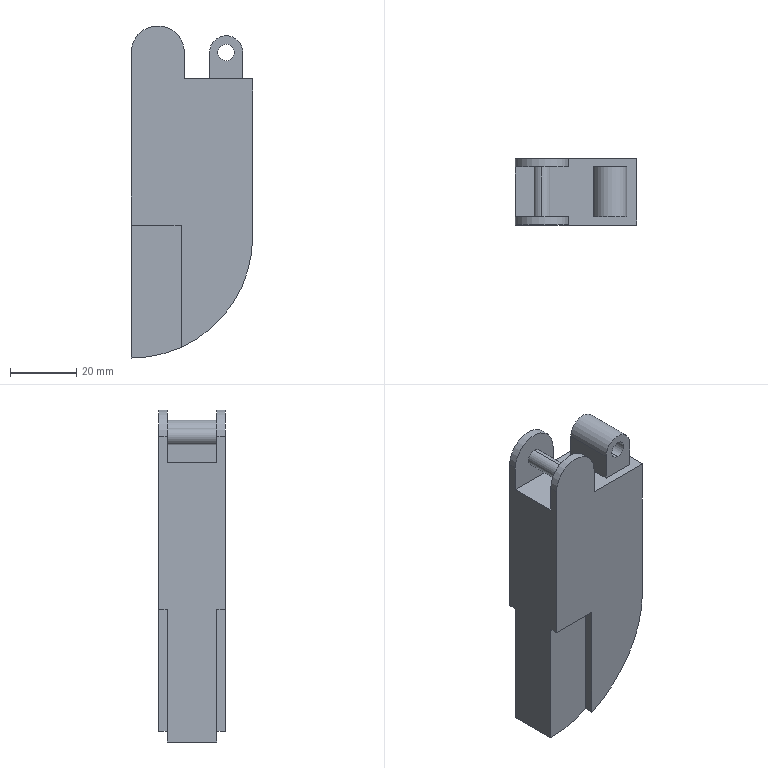Part | SolidWorks | 2 solids | 28 faces | box 36.56 x 20 x 100 mm | volume 55695 mm3 | plane 20 | cylinder 8 | commonest cylinder face diameters 5 x4 16 x2 10 x1 73.12 x1
STEP:
#1=CARTESIAN_POINT('',(8.,-7.5,-5.5));
#2=VERTEX_POINT('',#1);
#3=CARTESIAN_POINT('',(8.,-7.5,-10.5));
#4=VERTEX_POINT('',#3);
#5=CARTESIAN_POINT('',(8.,-7.5,-8.));
#6=DIRECTION('',(0.,1.,0.));
#7=DIRECTION('',(0.,0.,1.));
#8=AXIS2_PLACEMENT_3D('',#5,#6,#7);
#9=CIRCLE('',#8,2.5);
#10=EDGE_CURVE('',#2,#4,#9,.T.);
#11=ORIENTED_EDGE('',*,*,#10,.T.);
#12=CARTESIAN_POINT('',(8.,7.5,-10.5));
#13=VERTEX_POINT('',#12);
#14=CARTESIAN_POINT('',(8.,-17.071,-10.5));
#15=DIRECTION('',(0.,1.,0.));
#16=VECTOR('',#15,1000.);
#17=LINE('',#14,#16);
#18=EDGE_CURVE('',#4,#13,#17,.T.);
#19=ORIENTED_EDGE('',*,*,#18,.T.);
#20=CARTESIAN_POINT('',(8.,7.5,-5.5));
#21=VERTEX_POINT('',#20);
#22=CARTESIAN_POINT('',(8.,7.5,-8.));
#23=DIRECTION('',(0.,1.,0.));
#24=DIRECTION('',(0.,0.,1.));
#25=AXIS2_PLACEMENT_3D('',#22,#23,#24);
#26=CIRCLE('',#25,2.5);
#27=EDGE_CURVE('',#21,#13,#26,.T.);
#28=ORIENTED_EDGE('',*,*,#27,.F.);
#29=CARTESIAN_POINT('',(8.,-17.071,-5.5));
#30=DIRECTION('',(0.,1.,0.));
#31=VECTOR('',#30,1000.);
#32=LINE('',#29,#31);
#33=EDGE_CURVE('',#2,#21,#32,.T.);
#34=ORIENTED_EDGE('',*,*,#33,.F.);
#35=EDGE_LOOP('',(#11,#19,#28,#34));
#36=FACE_OUTER_BOUND('',#35,.T.);
#37=CARTESIAN_POINT('',(8.,-17.071,-8.));
#38=DIRECTION('',(0.,1.,0.));
#39=DIRECTION('',(0.,0.,1.));
#40=AXIS2_PLACEMENT_3D('',#37,#38,#39);
#41=CYLINDRICAL_SURFACE('',#40,2.5);
#42=ADVANCED_FACE('',(#36),#41,.T.);
#43=CARTESIAN_POINT('',(0.,10.,-8.));
#44=VERTEX_POINT('',#43);
#45=CARTESIAN_POINT('',(16.,10.,-8.));
#46=VERTEX_POINT('',#45);
#47=CARTESIAN_POINT('',(8.,10.,-8.));
#48=DIRECTION('',(0.,1.,0.));
#49=DIRECTION('',(0.,0.,1.));
#50=AXIS2_PLACEMENT_3D('',#47,#48,#49);
#51=CIRCLE('',#50,8.);
#52=EDGE_CURVE('',#44,#46,#51,.T.);
#53=ORIENTED_EDGE('',*,*,#52,.T.);
#54=CARTESIAN_POINT('',(16.,10.,-16.));
#55=VERTEX_POINT('',#54);
#56=CARTESIAN_POINT('',(16.,10.,-63.44));
#57=DIRECTION('',(0.,0.,1.));
#58=VECTOR('',#57,1000.);
#59=LINE('',#56,#58);
#60=EDGE_CURVE('',#55,#46,#59,.T.);
#61=ORIENTED_EDGE('',*,*,#60,.F.);
#62=CARTESIAN_POINT('',(36.56,10.,-16.));
#63=VERTEX_POINT('',#62);
#64=CARTESIAN_POINT('',(0.,10.,-16.));
#65=DIRECTION('',(-1.,0.,0.));
#66=VECTOR('',#65,1000.);
#67=LINE('',#64,#66);
#68=EDGE_CURVE('',#63,#55,#67,.T.);
#69=ORIENTED_EDGE('',*,*,#68,.F.);
#70=CARTESIAN_POINT('',(36.56,10.,-63.44));
#71=VERTEX_POINT('',#70);
#72=CARTESIAN_POINT('',(36.56,10.,0.));
#73=DIRECTION('',(0.,0.,-1.));
#74=VECTOR('',#73,1000.);
#75=LINE('',#72,#74);
#76=EDGE_CURVE('',#63,#71,#75,.T.);
#77=ORIENTED_EDGE('',*,*,#76,.T.);
#78=CARTESIAN_POINT('',(15.,10.,-96.781));
#79=VERTEX_POINT('',#78);
#80=CARTESIAN_POINT('',(0.,10.,-63.44));
#81=DIRECTION('',(0.,1.,0.));
#82=DIRECTION('',(0.,0.,1.));
#83=AXIS2_PLACEMENT_3D('',#80,#81,#82);
#84=CIRCLE('',#83,36.56);
#85=EDGE_CURVE('',#71,#79,#84,.T.);
#86=ORIENTED_EDGE('',*,*,#85,.T.);
#87=CARTESIAN_POINT('',(15.,10.,-60.));
#88=VERTEX_POINT('',#87);
#89=CARTESIAN_POINT('',(15.,10.,-100.));
#90=DIRECTION('',(0.,0.,-1.));
#91=VECTOR('',#90,1000.);
#92=LINE('',#89,#91);
#93=EDGE_CURVE('',#88,#79,#92,.T.);
#94=ORIENTED_EDGE('',*,*,#93,.F.);
#95=CARTESIAN_POINT('',(0.,10.,-60.));
#96=VERTEX_POINT('',#95);
#97=CARTESIAN_POINT('',(15.,10.,-60.));
#98=DIRECTION('',(-1.,0.,0.));
#99=VECTOR('',#98,1000.);
#100=LINE('',#97,#99);
#101=EDGE_CURVE('',#88,#96,#100,.T.);
#102=ORIENTED_EDGE('',*,*,#101,.T.);
#103=CARTESIAN_POINT('',(0.,10.,0.));
#104=DIRECTION('',(0.,0.,1.));
#105=VECTOR('',#104,1000.);
#106=LINE('',#103,#105);
#107=EDGE_CURVE('',#96,#44,#106,.T.);
#108=ORIENTED_EDGE('',*,*,#107,.T.);
#109=EDGE_LOOP('',(#53,#61,#69,#77,#86,#94,#102,#108));
#110=FACE_OUTER_BOUND('',#109,.T.);
#111=CARTESIAN_POINT('',(0.,10.,-63.44));
#112=DIRECTION('',(0.,1.,0.));
#113=DIRECTION('',(0.,0.,1.));
#114=AXIS2_PLACEMENT_3D('',#111,#112,#113);
#115=PLANE('',#114);
#116=ADVANCED_FACE('',(#110),#115,.T.);
#117=CARTESIAN_POINT('',(16.,-10.,-16.));
#118=VERTEX_POINT('',#117);
#119=CARTESIAN_POINT('',(16.,-10.,-8.));
#120=VERTEX_POINT('',#119);
#121=CARTESIAN_POINT('',(16.,-10.,-63.44));
#122=DIRECTION('',(0.,0.,1.));
#123=VECTOR('',#122,1000.);
#124=LINE('',#121,#123);
#125=EDGE_CURVE('',#118,#120,#124,.T.);
#126=ORIENTED_EDGE('',*,*,#125,.T.);
#127=CARTESIAN_POINT('',(0.,-10.,-8.));
#128=VERTEX_POINT('',#127);
#129=CARTESIAN_POINT('',(8.,-10.,-8.));
#130=DIRECTION('',(0.,-1.,0.));
#131=DIRECTION('',(0.,0.,1.));
#132=AXIS2_PLACEMENT_3D('',#129,#130,#131);
#133=CIRCLE('',#132,8.);
#134=EDGE_CURVE('',#120,#128,#133,.T.);
#135=ORIENTED_EDGE('',*,*,#134,.T.);
#136=CARTESIAN_POINT('',(0.,-10.,-60.));
#137=VERTEX_POINT('',#136);
#138=CARTESIAN_POINT('',(0.,-10.,0.));
#139=DIRECTION('',(0.,0.,1.));
#140=VECTOR('',#139,1000.);
#141=LINE('',#138,#140);
#142=EDGE_CURVE('',#137,#128,#141,.T.);
#143=ORIENTED_EDGE('',*,*,#142,.F.);
#144=CARTESIAN_POINT('',(15.,-10.,-60.));
#145=VERTEX_POINT('',#144);
#146=CARTESIAN_POINT('',(15.,-10.,-60.));
#147=DIRECTION('',(-1.,0.,0.));
#148=VECTOR('',#147,1000.);
#149=LINE('',#146,#148);
#150=EDGE_CURVE('',#145,#137,#149,.T.);
#151=ORIENTED_EDGE('',*,*,#150,.F.);
#152=CARTESIAN_POINT('',(15.,-10.,-96.781));
#153=VERTEX_POINT('',#152);
#154=CARTESIAN_POINT('',(15.,-10.,-63.44));
#155=DIRECTION('',(0.,0.,1.));
#156=VECTOR('',#155,1000.);
#157=LINE('',#154,#156);
#158=EDGE_CURVE('',#153,#145,#157,.T.);
#159=ORIENTED_EDGE('',*,*,#158,.F.);
#160=CARTESIAN_POINT('',(36.56,-10.,-63.44));
#161=VERTEX_POINT('',#160);
#162=CARTESIAN_POINT('',(0.,-10.,-63.44));
#163=DIRECTION('',(0.,1.,0.));
#164=DIRECTION('',(0.,0.,1.));
#165=AXIS2_PLACEMENT_3D('',#162,#163,#164);
#166=CIRCLE('',#165,36.56);
#167=EDGE_CURVE('',#161,#153,#166,.T.);
#168=ORIENTED_EDGE('',*,*,#167,.F.);
#169=CARTESIAN_POINT('',(36.56,-10.,-16.));
#170=VERTEX_POINT('',#169);
#171=CARTESIAN_POINT('',(36.56,-10.,0.));
#172=DIRECTION('',(0.,0.,-1.));
#173=VECTOR('',#172,1000.);
#174=LINE('',#171,#173);
#175=EDGE_CURVE('',#170,#161,#174,.T.);
#176=ORIENTED_EDGE('',*,*,#175,.F.);
#177=CARTESIAN_POINT('',(0.,-10.,-16.));
#178=DIRECTION('',(-1.,0.,0.));
#179=VECTOR('',#178,1000.);
#180=LINE('',#177,#179);
#181=EDGE_CURVE('',#170,#118,#180,.T.);
#182=ORIENTED_EDGE('',*,*,#181,.T.);
#183=EDGE_LOOP('',(#126,#135,#143,#151,#159,#168,#176,#182));
#184=FACE_OUTER_BOUND('',#183,.T.);
#185=CARTESIAN_POINT('',(0.,-10.,-63.44));
#186=DIRECTION('',(0.,1.,0.));
#187=DIRECTION('',(0.,0.,1.));
#188=AXIS2_PLACEMENT_3D('',#185,#186,#187);
#189=PLANE('',#188);
#190=ADVANCED_FACE('',(#184),#189,.F.);
#191=CARTESIAN_POINT('',(0.,-7.5,-8.));
#192=VERTEX_POINT('',#191);
#193=CARTESIAN_POINT('',(16.,-7.5,-8.));
#194=VERTEX_POINT('',#193);
#195=CARTESIAN_POINT('',(8.,-7.5,-8.));
#196=DIRECTION('',(0.,1.,0.));
#197=DIRECTION('',(0.,0.,1.));
#198=AXIS2_PLACEMENT_3D('',#195,#196,#197);
#199=CIRCLE('',#198,8.);
#200=EDGE_CURVE('',#192,#194,#199,.T.);
#201=ORIENTED_EDGE('',*,*,#200,.T.);
#202=CARTESIAN_POINT('',(16.,-7.5,-16.));
#203=VERTEX_POINT('',#202);
#204=CARTESIAN_POINT('',(16.,-7.5,0.));
#205=DIRECTION('',(0.,0.,1.));
#206=VECTOR('',#205,1000.);
#207=LINE('',#204,#206);
#208=EDGE_CURVE('',#203,#194,#207,.T.);
#209=ORIENTED_EDGE('',*,*,#208,.F.);
#210=CARTESIAN_POINT('',(0.,-7.5,-16.));
#211=VERTEX_POINT('',#210);
#212=CARTESIAN_POINT('',(0.,-7.5,-16.));
#213=DIRECTION('',(1.,0.,0.));
#214=VECTOR('',#213,1000.);
#215=LINE('',#212,#214);
#216=EDGE_CURVE('',#211,#203,#215,.T.);
#217=ORIENTED_EDGE('',*,*,#216,.F.);
#218=CARTESIAN_POINT('',(0.,-7.5,0.));
#219=DIRECTION('',(0.,0.,-1.));
#220=VECTOR('',#219,1000.);
#221=LINE('',#218,#220);
#222=EDGE_CURVE('',#192,#211,#221,.T.);
#223=ORIENTED_EDGE('',*,*,#222,.F.);
#224=EDGE_LOOP('',(#201,#209,#217,#223));
#225=FACE_OUTER_BOUND('',#224,.T.);
#226=ORIENTED_EDGE('',*,*,#10,.F.);
#227=CARTESIAN_POINT('',(8.,-7.5,-8.));
#228=DIRECTION('',(0.,1.,0.));
#229=DIRECTION('',(0.,0.,1.));
#230=AXIS2_PLACEMENT_3D('',#227,#228,#229);
#231=CIRCLE('',#230,2.5);
#232=EDGE_CURVE('',#4,#2,#231,.T.);
#233=ORIENTED_EDGE('',*,*,#232,.F.);
#234=EDGE_LOOP('',(#226,#233));
#235=FACE_BOUND('',#234,.T.);
#236=CARTESIAN_POINT('',(0.,-7.5,0.));
#237=DIRECTION('',(0.,1.,0.));
#238=DIRECTION('',(0.,0.,1.));
#239=AXIS2_PLACEMENT_3D('',#236,#237,#238);
#240=PLANE('',#239);
#241=ADVANCED_FACE('',(#225,#235),#240,.T.);
#242=ORIENTED_EDGE('',*,*,#27,.T.);
#243=CARTESIAN_POINT('',(8.,7.5,-8.));
#244=DIRECTION('',(0.,1.,0.));
#245=DIRECTION('',(0.,0.,1.));
#246=AXIS2_PLACEMENT_3D('',#243,#244,#245);
#247=CIRCLE('',#246,2.5);
#248=EDGE_CURVE('',#13,#21,#247,.T.);
#249=ORIENTED_EDGE('',*,*,#248,.T.);
#250=EDGE_LOOP('',(#242,#249));
#251=FACE_BOUND('',#250,.T.);
#252=CARTESIAN_POINT('',(16.,7.5,-16.));
#253=VERTEX_POINT('',#252);
#254=CARTESIAN_POINT('',(16.,7.5,-8.));
#255=VERTEX_POINT('',#254);
#256=CARTESIAN_POINT('',(16.,7.5,0.));
#257=DIRECTION('',(0.,0.,1.));
#258=VECTOR('',#257,1000.);
#259=LINE('',#256,#258);
#260=EDGE_CURVE('',#253,#255,#259,.T.);
#261=ORIENTED_EDGE('',*,*,#260,.T.);
#262=CARTESIAN_POINT('',(0.,7.5,-8.));
#263=VERTEX_POINT('',#262);
#264=CARTESIAN_POINT('',(8.,7.5,-8.));
#265=DIRECTION('',(0.,1.,0.));
#266=DIRECTION('',(0.,0.,1.));
#267=AXIS2_PLACEMENT_3D('',#264,#265,#266);
#268=CIRCLE('',#267,8.);
#269=EDGE_CURVE('',#263,#255,#268,.T.);
#270=ORIENTED_EDGE('',*,*,#269,.F.);
#271=CARTESIAN_POINT('',(0.,7.5,-16.));
#272=VERTEX_POINT('',#271);
#273=CARTESIAN_POINT('',(0.,7.5,0.));
#274=DIRECTION('',(0.,0.,-1.));
#275=VECTOR('',#274,1000.);
#276=LINE('',#273,#275);
#277=EDGE_CURVE('',#263,#272,#276,.T.);
#278=ORIENTED_EDGE('',*,*,#277,.T.);
#279=CARTESIAN_POINT('',(0.,7.5,-16.));
#280=DIRECTION('',(1.,0.,0.));
#281=VECTOR('',#280,1000.);
#282=LINE('',#279,#281);
#283=EDGE_CURVE('',#272,#253,#282,.T.);
#284=ORIENTED_EDGE('',*,*,#283,.T.);
#285=EDGE_LOOP('',(#261,#270,#278,#284));
#286=FACE_OUTER_BOUND('',#285,.T.);
#287=CARTESIAN_POINT('',(0.,7.5,0.));
#288=DIRECTION('',(0.,1.,0.));
#289=DIRECTION('',(0.,0.,1.));
#290=AXIS2_PLACEMENT_3D('',#287,#288,#289);
#291=PLANE('',#290);
#292=ADVANCED_FACE('',(#251,#286),#291,.F.);
#293=ORIENTED_EDGE('',*,*,#76,.F.);
#294=CARTESIAN_POINT('',(36.56,-7.5,-16.));
#295=DIRECTION('',(0.,1.,0.));
#296=VECTOR('',#295,1000.);
#297=LINE('',#294,#296);
#298=EDGE_CURVE('',#170,#63,#297,.T.);
#299=ORIENTED_EDGE('',*,*,#298,.F.);
#300=ORIENTED_EDGE('',*,*,#175,.T.);
#301=CARTESIAN_POINT('',(36.56,10.,-63.44));
#302=DIRECTION('',(0.,-1.,0.));
#303=VECTOR('',#302,1000.);
#304=LINE('',#301,#303);
#305=EDGE_CURVE('',#71,#161,#304,.T.);
#306=ORIENTED_EDGE('',*,*,#305,.F.);
#307=EDGE_LOOP('',(#293,#299,#300,#306));
#308=FACE_OUTER_BOUND('',#307,.T.);
#309=CARTESIAN_POINT('',(36.56,10.,0.));
#310=DIRECTION('',(-1.,0.,0.));
#311=DIRECTION('',(0.,0.,1.));
#312=AXIS2_PLACEMENT_3D('',#309,#310,#311);
#313=PLANE('',#312);
#314=ADVANCED_FACE('',(#308),#313,.F.);
#315=ORIENTED_EDGE('',*,*,#222,.T.);
#316=CARTESIAN_POINT('',(0.,-7.5,-16.));
#317=DIRECTION('',(0.,1.,0.));
#318=VECTOR('',#317,1000.);
#319=LINE('',#316,#318);
#320=EDGE_CURVE('',#211,#272,#319,.T.);
#321=ORIENTED_EDGE('',*,*,#320,.T.);
#322=ORIENTED_EDGE('',*,*,#277,.F.);
#323=CARTESIAN_POINT('',(0.,10.,-8.));
#324=DIRECTION('',(0.,1.,0.));
#325=VECTOR('',#324,1000.);
#326=LINE('',#323,#325);
#327=EDGE_CURVE('',#263,#44,#326,.T.);
#328=ORIENTED_EDGE('',*,*,#327,.T.);
#329=ORIENTED_EDGE('',*,*,#107,.F.);
#330=CARTESIAN_POINT('',(0.,7.5,-60.));
#331=VERTEX_POINT('',#330);
#332=CARTESIAN_POINT('',(0.,10.,-60.));
#333=DIRECTION('',(0.,1.,0.));
#334=VECTOR('',#333,1000.);
#335=LINE('',#332,#334);
#336=EDGE_CURVE('',#331,#96,#335,.T.);
#337=ORIENTED_EDGE('',*,*,#336,.F.);
#338=CARTESIAN_POINT('',(0.,7.5,-100.));
#339=VERTEX_POINT('',#338);
#340=CARTESIAN_POINT('',(0.,7.5,-100.));
#341=DIRECTION('',(0.,0.,1.));
#342=VECTOR('',#341,1000.);
#343=LINE('',#340,#342);
#344=EDGE_CURVE('',#339,#331,#343,.T.);
#345=ORIENTED_EDGE('',*,*,#344,.F.);
#346=CARTESIAN_POINT('',(0.,-7.5,-100.));
#347=VERTEX_POINT('',#346);
#348=CARTESIAN_POINT('',(0.,10.,-100.));
#349=DIRECTION('',(0.,-1.,0.));
#350=VECTOR('',#349,1000.);
#351=LINE('',#348,#350);
#352=EDGE_CURVE('',#339,#347,#351,.T.);
#353=ORIENTED_EDGE('',*,*,#352,.T.);
#354=CARTESIAN_POINT('',(0.,-7.5,-60.));
#355=VERTEX_POINT('',#354);
#356=CARTESIAN_POINT('',(0.,-7.5,-100.));
#357=DIRECTION('',(0.,0.,-1.));
#358=VECTOR('',#357,1000.);
#359=LINE('',#356,#358);
#360=EDGE_CURVE('',#355,#347,#359,.T.);
#361=ORIENTED_EDGE('',*,*,#360,.F.);
#362=CARTESIAN_POINT('',(0.,-10.,-60.));
#363=DIRECTION('',(0.,1.,0.));
#364=VECTOR('',#363,1000.);
#365=LINE('',#362,#364);
#366=EDGE_CURVE('',#137,#355,#365,.T.);
#367=ORIENTED_EDGE('',*,*,#366,.F.);
#368=ORIENTED_EDGE('',*,*,#142,.T.);
#369=CARTESIAN_POINT('',(0.,10.,-8.));
#370=DIRECTION('',(0.,1.,0.));
#371=VECTOR('',#370,1000.);
#372=LINE('',#369,#371);
#373=EDGE_CURVE('',#128,#192,#372,.T.);
#374=ORIENTED_EDGE('',*,*,#373,.T.);
#375=EDGE_LOOP('',(#315,#321,#322,#328,#329,#337,#345,#353,#361,#367,#368,#374));
#376=FACE_OUTER_BOUND('',#375,.T.);
#377=CARTESIAN_POINT('',(0.,10.,0.));
#378=DIRECTION('',(1.,0.,0.));
#379=DIRECTION('',(0.,0.,-1.));
#380=AXIS2_PLACEMENT_3D('',#377,#378,#379);
#381=PLANE('',#380);
#382=ADVANCED_FACE('',(#376),#381,.F.);
#383=ORIENTED_EDGE('',*,*,#373,.F.);
#384=ORIENTED_EDGE('',*,*,#134,.F.);
#385=CARTESIAN_POINT('',(16.,-30.,-8.));
#386=DIRECTION('',(0.,1.,0.));
#387=VECTOR('',#386,1000.);
#388=LINE('',#385,#387);
#389=EDGE_CURVE('',#120,#194,#388,.T.);
#390=ORIENTED_EDGE('',*,*,#389,.T.);
#391=ORIENTED_EDGE('',*,*,#200,.F.);
#392=EDGE_LOOP('',(#383,#384,#390,#391));
#393=FACE_OUTER_BOUND('',#392,.T.);
#394=CARTESIAN_POINT('',(8.,10.,-8.));
#395=DIRECTION('',(0.,-1.,0.));
#396=DIRECTION('',(0.,0.,-1.));
#397=AXIS2_PLACEMENT_3D('',#394,#395,#396);
#398=CYLINDRICAL_SURFACE('',#397,8.);
#399=ADVANCED_FACE('',(#393),#398,.T.);
#400=ORIENTED_EDGE('',*,*,#352,.F.);
#401=CARTESIAN_POINT('',(15.,7.5,-96.781));
#402=VERTEX_POINT('',#401);
#403=CARTESIAN_POINT('',(0.,7.5,-63.44));
#404=DIRECTION('',(0.,-1.,0.));
#405=DIRECTION('',(0.,0.,-1.));
#406=AXIS2_PLACEMENT_3D('',#403,#404,#405);
#407=CIRCLE('',#406,36.56);
#408=EDGE_CURVE('',#339,#402,#407,.T.);
#409=ORIENTED_EDGE('',*,*,#408,.T.);
#410=CARTESIAN_POINT('',(15.,10.,-96.781));
#411=DIRECTION('',(0.,-1.,0.));
#412=VECTOR('',#411,1000.);
#413=LINE('',#410,#412);
#414=EDGE_CURVE('',#79,#402,#413,.T.);
#415=ORIENTED_EDGE('',*,*,#414,.F.);
#416=ORIENTED_EDGE('',*,*,#85,.F.);
#417=ORIENTED_EDGE('',*,*,#305,.T.);
#418=ORIENTED_EDGE('',*,*,#167,.T.);
#419=CARTESIAN_POINT('',(15.,-7.5,-96.781));
#420=VERTEX_POINT('',#419);
#421=CARTESIAN_POINT('',(15.,10.,-96.781));
#422=DIRECTION('',(0.,-1.,0.));
#423=VECTOR('',#422,1000.);
#424=LINE('',#421,#423);
#425=EDGE_CURVE('',#420,#153,#424,.T.);
#426=ORIENTED_EDGE('',*,*,#425,.F.);
#427=CARTESIAN_POINT('',(0.,-7.5,-63.44));
#428=DIRECTION('',(0.,1.,0.));
#429=DIRECTION('',(0.,0.,1.));
#430=AXIS2_PLACEMENT_3D('',#427,#428,#429);
#431=CIRCLE('',#430,36.56);
#432=EDGE_CURVE('',#420,#347,#431,.T.);
#433=ORIENTED_EDGE('',*,*,#432,.T.);
#434=EDGE_LOOP('',(#400,#409,#415,#416,#417,#418,#426,#433));
#435=FACE_OUTER_BOUND('',#434,.T.);
#436=CARTESIAN_POINT('',(0.,10.,-63.44));
#437=DIRECTION('',(0.,-1.,0.));
#438=DIRECTION('',(0.,0.,-1.));
#439=AXIS2_PLACEMENT_3D('',#436,#437,#438);
#440=CYLINDRICAL_SURFACE('',#439,36.56);
#441=ADVANCED_FACE('',(#435),#440,.T.);
#442=CARTESIAN_POINT('',(15.,-7.5,-60.));
#443=VERTEX_POINT('',#442);
#444=CARTESIAN_POINT('',(15.,-7.5,-100.));
#445=DIRECTION('',(0.,0.,-1.));
#446=VECTOR('',#445,1000.);
#447=LINE('',#444,#446);
#448=EDGE_CURVE('',#443,#420,#447,.T.);
#449=ORIENTED_EDGE('',*,*,#448,.F.);
#450=CARTESIAN_POINT('',(15.,-7.5,-60.));
#451=DIRECTION('',(-1.,0.,0.));
#452=VECTOR('',#451,1000.);
#453=LINE('',#450,#452);
#454=EDGE_CURVE('',#443,#355,#453,.T.);
#455=ORIENTED_EDGE('',*,*,#454,.T.);
#456=ORIENTED_EDGE('',*,*,#360,.T.);
#457=ORIENTED_EDGE('',*,*,#432,.F.);
#458=EDGE_LOOP('',(#449,#455,#456,#457));
#459=FACE_OUTER_BOUND('',#458,.T.);
#460=CARTESIAN_POINT('',(15.,-7.5,-100.));
#461=DIRECTION('',(0.,1.,0.));
#462=DIRECTION('',(0.,0.,1.));
#463=AXIS2_PLACEMENT_3D('',#460,#461,#462);
#464=PLANE('',#463);
#465=ADVANCED_FACE('',(#459),#464,.F.);
#466=ORIENTED_EDGE('',*,*,#425,.T.);
#467=ORIENTED_EDGE('',*,*,#158,.T.);
#468=CARTESIAN_POINT('',(15.,-10.,-60.));
#469=DIRECTION('',(0.,1.,0.));
#470=VECTOR('',#469,1000.);
#471=LINE('',#468,#470);
#472=EDGE_CURVE('',#145,#443,#471,.T.);
#473=ORIENTED_EDGE('',*,*,#472,.T.);
#474=ORIENTED_EDGE('',*,*,#448,.T.);
#475=EDGE_LOOP('',(#466,#467,#473,#474));
#476=FACE_OUTER_BOUND('',#475,.T.);
#477=CARTESIAN_POINT('',(15.,0.,0.));
#478=DIRECTION('',(-1.,0.,0.));
#479=DIRECTION('',(0.,0.,1.));
#480=AXIS2_PLACEMENT_3D('',#477,#478,#479);
#481=PLANE('',#480);
#482=ADVANCED_FACE('',(#476),#481,.T.);
#483=ORIENTED_EDGE('',*,*,#366,.T.);
#484=ORIENTED_EDGE('',*,*,#454,.F.);
#485=ORIENTED_EDGE('',*,*,#472,.F.);
#486=ORIENTED_EDGE('',*,*,#150,.T.);
#487=EDGE_LOOP('',(#483,#484,#485,#486));
#488=FACE_OUTER_BOUND('',#487,.T.);
#489=CARTESIAN_POINT('',(15.,-10.,-60.));
#490=DIRECTION('',(0.,0.,1.));
#491=DIRECTION('',(0.,-1.,0.));
#492=AXIS2_PLACEMENT_3D('',#489,#490,#491);
#493=PLANE('',#492);
#494=ADVANCED_FACE('',(#488),#493,.F.);
#495=ORIENTED_EDGE('',*,*,#344,.T.);
#496=CARTESIAN_POINT('',(15.,7.5,-60.));
#497=VERTEX_POINT('',#496);
#498=CARTESIAN_POINT('',(15.,7.5,-60.));
#499=DIRECTION('',(-1.,0.,0.));
#500=VECTOR('',#499,1000.);
#501=LINE('',#498,#500);
#502=EDGE_CURVE('',#497,#331,#501,.T.);
#503=ORIENTED_EDGE('',*,*,#502,.F.);
#504=CARTESIAN_POINT('',(15.,7.5,-100.));
#505=DIRECTION('',(0.,0.,1.));
#506=VECTOR('',#505,1000.);
#507=LINE('',#504,#506);
#508=EDGE_CURVE('',#402,#497,#507,.T.);
#509=ORIENTED_EDGE('',*,*,#508,.F.);
#510=ORIENTED_EDGE('',*,*,#408,.F.);
#511=EDGE_LOOP('',(#495,#503,#509,#510));
#512=FACE_OUTER_BOUND('',#511,.T.);
#513=CARTESIAN_POINT('',(15.,7.5,-100.));
#514=DIRECTION('',(0.,-1.,0.));
#515=DIRECTION('',(0.,0.,-1.));
#516=AXIS2_PLACEMENT_3D('',#513,#514,#515);
#517=PLANE('',#516);
#518=ADVANCED_FACE('',(#512),#517,.F.);
#519=ORIENTED_EDGE('',*,*,#414,.T.);
#520=ORIENTED_EDGE('',*,*,#508,.T.);
#521=CARTESIAN_POINT('',(15.,10.,-60.));
#522=DIRECTION('',(0.,1.,0.));
#523=VECTOR('',#522,1000.);
#524=LINE('',#521,#523);
#525=EDGE_CURVE('',#497,#88,#524,.T.);
#526=ORIENTED_EDGE('',*,*,#525,.T.);
#527=ORIENTED_EDGE('',*,*,#93,.T.);
#528=EDGE_LOOP('',(#519,#520,#526,#527));
#529=FACE_OUTER_BOUND('',#528,.T.);
#530=CARTESIAN_POINT('',(15.,0.,0.));
#531=DIRECTION('',(-1.,0.,0.));
#532=DIRECTION('',(0.,0.,1.));
#533=AXIS2_PLACEMENT_3D('',#530,#531,#532);
#534=PLANE('',#533);
#535=ADVANCED_FACE('',(#529),#534,.T.);
#536=ORIENTED_EDGE('',*,*,#336,.T.);
#537=ORIENTED_EDGE('',*,*,#101,.F.);
#538=ORIENTED_EDGE('',*,*,#525,.F.);
#539=ORIENTED_EDGE('',*,*,#502,.T.);
#540=EDGE_LOOP('',(#536,#537,#538,#539));
#541=FACE_OUTER_BOUND('',#540,.T.);
#542=CARTESIAN_POINT('',(15.,10.,-60.));
#543=DIRECTION('',(0.,0.,1.));
#544=DIRECTION('',(0.,-1.,0.));
#545=AXIS2_PLACEMENT_3D('',#542,#543,#544);
#546=PLANE('',#545);
#547=ADVANCED_FACE('',(#541),#546,.F.);
#548=ORIENTED_EDGE('',*,*,#269,.T.);
#549=CARTESIAN_POINT('',(16.,-30.,-8.));
#550=DIRECTION('',(0.,1.,0.));
#551=VECTOR('',#550,1000.);
#552=LINE('',#549,#551);
#553=EDGE_CURVE('',#255,#46,#552,.T.);
#554=ORIENTED_EDGE('',*,*,#553,.T.);
#555=ORIENTED_EDGE('',*,*,#52,.F.);
#556=ORIENTED_EDGE('',*,*,#327,.F.);
#557=EDGE_LOOP('',(#548,#554,#555,#556));
#558=FACE_OUTER_BOUND('',#557,.T.);
#559=CARTESIAN_POINT('',(8.,10.,-8.));
#560=DIRECTION('',(0.,-1.,0.));
#561=DIRECTION('',(0.,0.,-1.));
#562=AXIS2_PLACEMENT_3D('',#559,#560,#561);
#563=CYLINDRICAL_SURFACE('',#562,8.);
#564=ADVANCED_FACE('',(#558),#563,.T.);
#565=ORIENTED_EDGE('',*,*,#216,.T.);
#566=CARTESIAN_POINT('',(16.,-30.,-16.));
#567=DIRECTION('',(0.,1.,0.));
#568=VECTOR('',#567,1000.);
#569=LINE('',#566,#568);
#570=EDGE_CURVE('',#118,#203,#569,.T.);
#571=ORIENTED_EDGE('',*,*,#570,.F.);
#572=ORIENTED_EDGE('',*,*,#181,.F.);
#573=ORIENTED_EDGE('',*,*,#298,.T.);
#574=ORIENTED_EDGE('',*,*,#68,.T.);
#575=CARTESIAN_POINT('',(16.,-30.,-16.));
#576=DIRECTION('',(0.,1.,0.));
#577=VECTOR('',#576,1000.);
#578=LINE('',#575,#577);
#579=EDGE_CURVE('',#253,#55,#578,.T.);
#580=ORIENTED_EDGE('',*,*,#579,.F.);
#581=ORIENTED_EDGE('',*,*,#283,.F.);
#582=ORIENTED_EDGE('',*,*,#320,.F.);
#583=EDGE_LOOP('',(#565,#571,#572,#573,#574,#580,#581,#582));
#584=FACE_OUTER_BOUND('',#583,.T.);
#585=CARTESIAN_POINT('',(0.,-7.5,-16.));
#586=DIRECTION('',(0.,0.,1.));
#587=DIRECTION('',(1.,0.,0.));
#588=AXIS2_PLACEMENT_3D('',#585,#586,#587);
#589=PLANE('',#588);
#590=ADVANCED_FACE('',(#584),#589,.T.);
#591=ORIENTED_EDGE('',*,*,#18,.F.);
#592=ORIENTED_EDGE('',*,*,#232,.T.);
#593=ORIENTED_EDGE('',*,*,#33,.T.);
#594=ORIENTED_EDGE('',*,*,#248,.F.);
#595=EDGE_LOOP('',(#591,#592,#593,#594));
#596=FACE_OUTER_BOUND('',#595,.T.);
#597=CARTESIAN_POINT('',(8.,-17.071,-8.));
#598=DIRECTION('',(0.,1.,0.));
#599=DIRECTION('',(0.,0.,1.));
#600=AXIS2_PLACEMENT_3D('',#597,#598,#599);
#601=CYLINDRICAL_SURFACE('',#600,2.5);
#602=ADVANCED_FACE('',(#596),#601,.T.);
#603=ORIENTED_EDGE('',*,*,#570,.T.);
#604=ORIENTED_EDGE('',*,*,#208,.T.);
#605=ORIENTED_EDGE('',*,*,#389,.F.);
#606=ORIENTED_EDGE('',*,*,#125,.F.);
#607=EDGE_LOOP('',(#603,#604,#605,#606));
#608=FACE_OUTER_BOUND('',#607,.T.);
#609=CARTESIAN_POINT('',(16.,-30.,-8.));
#610=DIRECTION('',(-1.,0.,0.));
#611=DIRECTION('',(0.,0.,1.));
#612=AXIS2_PLACEMENT_3D('',#609,#610,#611);
#613=PLANE('',#612);
#614=ADVANCED_FACE('',(#608),#613,.F.);
#615=ORIENTED_EDGE('',*,*,#60,.T.);
#616=ORIENTED_EDGE('',*,*,#553,.F.);
#617=ORIENTED_EDGE('',*,*,#260,.F.);
#618=ORIENTED_EDGE('',*,*,#579,.T.);
#619=EDGE_LOOP('',(#615,#616,#617,#618));
#620=FACE_OUTER_BOUND('',#619,.T.);
#621=CARTESIAN_POINT('',(16.,-30.,-8.));
#622=DIRECTION('',(-1.,0.,0.));
#623=DIRECTION('',(0.,0.,1.));
#624=AXIS2_PLACEMENT_3D('',#621,#622,#623);
#625=PLANE('',#624);
#626=ADVANCED_FACE('',(#620),#625,.F.);
#627=CLOSED_SHELL('',(#42,#116,#190,#241,#292,#314,#382,#399,#441,#465,#482,#494,#518,#535,#547,#564,#590,#602,#614,#626));
#628=MANIFOLD_SOLID_BREP('',#627);
#629=CARTESIAN_POINT('',(28.56,7.5,-10.5));
#630=VERTEX_POINT('',#629);
#631=CARTESIAN_POINT('',(28.56,7.5,-5.5));
#632=VERTEX_POINT('',#631);
#633=CARTESIAN_POINT('',(28.56,7.5,-8.));
#634=DIRECTION('',(0.,1.,0.));
#635=DIRECTION('',(0.,0.,1.));
#636=AXIS2_PLACEMENT_3D('',#633,#634,#635);
#637=CIRCLE('',#636,2.5);
#638=EDGE_CURVE('',#630,#632,#637,.T.);
#639=ORIENTED_EDGE('',*,*,#638,.T.);
#640=CARTESIAN_POINT('',(28.56,-7.5,-5.5));
#641=VERTEX_POINT('',#640);
#642=CARTESIAN_POINT('',(28.56,7.5,-5.5));
#643=DIRECTION('',(0.,-1.,0.));
#644=VECTOR('',#643,1000.);
#645=LINE('',#642,#644);
#646=EDGE_CURVE('',#632,#641,#645,.T.);
#647=ORIENTED_EDGE('',*,*,#646,.T.);
#648=CARTESIAN_POINT('',(28.56,-7.5,-10.5));
#649=VERTEX_POINT('',#648);
#650=CARTESIAN_POINT('',(28.56,-7.5,-8.));
#651=DIRECTION('',(0.,1.,0.));
#652=DIRECTION('',(0.,0.,1.));
#653=AXIS2_PLACEMENT_3D('',#650,#651,#652);
#654=CIRCLE('',#653,2.5);
#655=EDGE_CURVE('',#649,#641,#654,.T.);
#656=ORIENTED_EDGE('',*,*,#655,.F.);
#657=CARTESIAN_POINT('',(28.56,7.5,-10.5));
#658=DIRECTION('',(0.,-1.,0.));
#659=VECTOR('',#658,1000.);
#660=LINE('',#657,#659);
#661=EDGE_CURVE('',#630,#649,#660,.T.);
#662=ORIENTED_EDGE('',*,*,#661,.F.);
#663=EDGE_LOOP('',(#639,#647,#656,#662));
#664=FACE_OUTER_BOUND('',#663,.T.);
#665=CARTESIAN_POINT('',(28.56,7.5,-8.));
#666=DIRECTION('',(0.,-1.,0.));
#667=DIRECTION('',(0.,0.,-1.));
#668=AXIS2_PLACEMENT_3D('',#665,#666,#667);
#669=CYLINDRICAL_SURFACE('',#668,2.5);
#670=ADVANCED_FACE('',(#664),#669,.F.);
#671=CARTESIAN_POINT('',(23.56,7.5,-8.));
#672=VERTEX_POINT('',#671);
#673=CARTESIAN_POINT('',(23.56,7.5,-16.));
#674=VERTEX_POINT('',#673);
#675=CARTESIAN_POINT('',(23.56,7.5,-8.));
#676=DIRECTION('',(0.,0.,-1.));
#677=VECTOR('',#676,1000.);
#678=LINE('',#675,#677);
#679=EDGE_CURVE('',#672,#674,#678,.T.);
#680=ORIENTED_EDGE('',*,*,#679,.F.);
#681=CARTESIAN_POINT('',(33.56,7.5,-8.));
#682=VERTEX_POINT('',#681);
#683=CARTESIAN_POINT('',(28.56,7.5,-8.));
#684=DIRECTION('',(0.,1.,0.));
#685=DIRECTION('',(0.,0.,1.));
#686=AXIS2_PLACEMENT_3D('',#683,#684,#685);
#687=CIRCLE('',#686,5.);
#688=EDGE_CURVE('',#672,#682,#687,.T.);
#689=ORIENTED_EDGE('',*,*,#688,.T.);
#690=CARTESIAN_POINT('',(33.56,7.5,-16.));
#691=VERTEX_POINT('',#690);
#692=CARTESIAN_POINT('',(33.56,7.5,-16.));
#693=DIRECTION('',(0.,0.,1.));
#694=VECTOR('',#693,1000.);
#695=LINE('',#692,#694);
#696=EDGE_CURVE('',#691,#682,#695,.T.);
#697=ORIENTED_EDGE('',*,*,#696,.F.);
#698=CARTESIAN_POINT('',(23.56,7.5,-16.));
#699=DIRECTION('',(1.,0.,0.));
#700=VECTOR('',#699,1000.);
#701=LINE('',#698,#700);
#702=EDGE_CURVE('',#674,#691,#701,.T.);
#703=ORIENTED_EDGE('',*,*,#702,.F.);
#704=EDGE_LOOP('',(#680,#689,#697,#703));
#705=FACE_OUTER_BOUND('',#704,.T.);
#706=ORIENTED_EDGE('',*,*,#638,.F.);
#707=CARTESIAN_POINT('',(28.56,7.5,-8.));
#708=DIRECTION('',(0.,1.,0.));
#709=DIRECTION('',(0.,0.,1.));
#710=AXIS2_PLACEMENT_3D('',#707,#708,#709);
#711=CIRCLE('',#710,2.5);
#712=EDGE_CURVE('',#632,#630,#711,.T.);
#713=ORIENTED_EDGE('',*,*,#712,.F.);
#714=EDGE_LOOP('',(#706,#713));
#715=FACE_BOUND('',#714,.T.);
#716=CARTESIAN_POINT('',(28.56,7.5,-8.));
#717=DIRECTION('',(0.,1.,0.));
#718=DIRECTION('',(0.,0.,1.));
#719=AXIS2_PLACEMENT_3D('',#716,#717,#718);
#720=PLANE('',#719);
#721=ADVANCED_FACE('',(#705,#715),#720,.T.);
#722=CARTESIAN_POINT('',(23.56,-7.5,-8.));
#723=VERTEX_POINT('',#722);
#724=CARTESIAN_POINT('',(23.56,-7.5,-16.));
#725=VERTEX_POINT('',#724);
#726=CARTESIAN_POINT('',(23.56,-7.5,-8.));
#727=DIRECTION('',(0.,0.,-1.));
#728=VECTOR('',#727,1000.);
#729=LINE('',#726,#728);
#730=EDGE_CURVE('',#723,#725,#729,.T.);
#731=ORIENTED_EDGE('',*,*,#730,.T.);
#732=CARTESIAN_POINT('',(33.56,-7.5,-16.));
#733=VERTEX_POINT('',#732);
#734=CARTESIAN_POINT('',(23.56,-7.5,-16.));
#735=DIRECTION('',(1.,0.,0.));
#736=VECTOR('',#735,1000.);
#737=LINE('',#734,#736);
#738=EDGE_CURVE('',#725,#733,#737,.T.);
#739=ORIENTED_EDGE('',*,*,#738,.T.);
#740=CARTESIAN_POINT('',(33.56,-7.5,-8.));
#741=VERTEX_POINT('',#740);
#742=CARTESIAN_POINT('',(33.56,-7.5,-16.));
#743=DIRECTION('',(0.,0.,1.));
#744=VECTOR('',#743,1000.);
#745=LINE('',#742,#744);
#746=EDGE_CURVE('',#733,#741,#745,.T.);
#747=ORIENTED_EDGE('',*,*,#746,.T.);
#748=CARTESIAN_POINT('',(28.56,-7.5,-8.));
#749=DIRECTION('',(0.,1.,0.));
#750=DIRECTION('',(0.,0.,1.));
#751=AXIS2_PLACEMENT_3D('',#748,#749,#750);
#752=CIRCLE('',#751,5.);
#753=EDGE_CURVE('',#723,#741,#752,.T.);
#754=ORIENTED_EDGE('',*,*,#753,.F.);
#755=EDGE_LOOP('',(#731,#739,#747,#754));
#756=FACE_OUTER_BOUND('',#755,.T.);
#757=ORIENTED_EDGE('',*,*,#655,.T.);
#758=CARTESIAN_POINT('',(28.56,-7.5,-8.));
#759=DIRECTION('',(0.,1.,0.));
#760=DIRECTION('',(0.,0.,1.));
#761=AXIS2_PLACEMENT_3D('',#758,#759,#760);
#762=CIRCLE('',#761,2.5);
#763=EDGE_CURVE('',#641,#649,#762,.T.);
#764=ORIENTED_EDGE('',*,*,#763,.T.);
#765=EDGE_LOOP('',(#757,#764));
#766=FACE_BOUND('',#765,.T.);
#767=CARTESIAN_POINT('',(28.56,-7.5,-8.));
#768=DIRECTION('',(0.,1.,0.));
#769=DIRECTION('',(0.,0.,1.));
#770=AXIS2_PLACEMENT_3D('',#767,#768,#769);
#771=PLANE('',#770);
#772=ADVANCED_FACE('',(#756,#766),#771,.F.);
#773=ORIENTED_EDGE('',*,*,#730,.F.);
#774=CARTESIAN_POINT('',(23.56,7.5,-8.));
#775=DIRECTION('',(0.,-1.,0.));
#776=VECTOR('',#775,1000.);
#777=LINE('',#774,#776);
#778=EDGE_CURVE('',#672,#723,#777,.T.);
#779=ORIENTED_EDGE('',*,*,#778,.F.);
#780=ORIENTED_EDGE('',*,*,#679,.T.);
#781=CARTESIAN_POINT('',(23.56,7.5,-16.));
#782=DIRECTION('',(0.,-1.,0.));
#783=VECTOR('',#782,1000.);
#784=LINE('',#781,#783);
#785=EDGE_CURVE('',#674,#725,#784,.T.);
#786=ORIENTED_EDGE('',*,*,#785,.T.);
#787=EDGE_LOOP('',(#773,#779,#780,#786));
#788=FACE_OUTER_BOUND('',#787,.T.);
#789=CARTESIAN_POINT('',(23.56,7.5,-8.));
#790=DIRECTION('',(-1.,0.,0.));
#791=DIRECTION('',(0.,0.,1.));
#792=AXIS2_PLACEMENT_3D('',#789,#790,#791);
#793=PLANE('',#792);
#794=ADVANCED_FACE('',(#788),#793,.T.);
#795=ORIENTED_EDGE('',*,*,#753,.T.);
#796=CARTESIAN_POINT('',(33.56,7.5,-8.));
#797=DIRECTION('',(0.,-1.,0.));
#798=VECTOR('',#797,1000.);
#799=LINE('',#796,#798);
#800=EDGE_CURVE('',#682,#741,#799,.T.);
#801=ORIENTED_EDGE('',*,*,#800,.F.);
#802=ORIENTED_EDGE('',*,*,#688,.F.);
#803=ORIENTED_EDGE('',*,*,#778,.T.);
#804=EDGE_LOOP('',(#795,#801,#802,#803));
#805=FACE_OUTER_BOUND('',#804,.T.);
#806=CARTESIAN_POINT('',(28.56,7.5,-8.));
#807=DIRECTION('',(0.,-1.,0.));
#808=DIRECTION('',(0.,0.,-1.));
#809=AXIS2_PLACEMENT_3D('',#806,#807,#808);
#810=CYLINDRICAL_SURFACE('',#809,5.);
#811=ADVANCED_FACE('',(#805),#810,.T.);
#812=ORIENTED_EDGE('',*,*,#746,.F.);
#813=CARTESIAN_POINT('',(33.56,7.5,-16.));
#814=DIRECTION('',(0.,-1.,0.));
#815=VECTOR('',#814,1000.);
#816=LINE('',#813,#815);
#817=EDGE_CURVE('',#691,#733,#816,.T.);
#818=ORIENTED_EDGE('',*,*,#817,.F.);
#819=ORIENTED_EDGE('',*,*,#696,.T.);
#820=ORIENTED_EDGE('',*,*,#800,.T.);
#821=EDGE_LOOP('',(#812,#818,#819,#820));
#822=FACE_OUTER_BOUND('',#821,.T.);
#823=CARTESIAN_POINT('',(33.56,7.5,-16.));
#824=DIRECTION('',(1.,0.,0.));
#825=DIRECTION('',(0.,0.,-1.));
#826=AXIS2_PLACEMENT_3D('',#823,#824,#825);
#827=PLANE('',#826);
#828=ADVANCED_FACE('',(#822),#827,.T.);
#829=ORIENTED_EDGE('',*,*,#738,.F.);
#830=ORIENTED_EDGE('',*,*,#785,.F.);
#831=ORIENTED_EDGE('',*,*,#702,.T.);
#832=ORIENTED_EDGE('',*,*,#817,.T.);
#833=EDGE_LOOP('',(#829,#830,#831,#832));
#834=FACE_OUTER_BOUND('',#833,.T.);
#835=CARTESIAN_POINT('',(23.56,7.5,-16.));
#836=DIRECTION('',(0.,0.,-1.));
#837=DIRECTION('',(-1.,0.,0.));
#838=AXIS2_PLACEMENT_3D('',#835,#836,#837);
#839=PLANE('',#838);
#840=ADVANCED_FACE('',(#834),#839,.T.);
#841=ORIENTED_EDGE('',*,*,#646,.F.);
#842=ORIENTED_EDGE('',*,*,#712,.T.);
#843=ORIENTED_EDGE('',*,*,#661,.T.);
#844=ORIENTED_EDGE('',*,*,#763,.F.);
#845=EDGE_LOOP('',(#841,#842,#843,#844));
#846=FACE_OUTER_BOUND('',#845,.T.);
#847=CARTESIAN_POINT('',(28.56,7.5,-8.));
#848=DIRECTION('',(0.,-1.,0.));
#849=DIRECTION('',(0.,0.,-1.));
#850=AXIS2_PLACEMENT_3D('',#847,#848,#849);
#851=CYLINDRICAL_SURFACE('',#850,2.5);
#852=ADVANCED_FACE('',(#846),#851,.F.);
#853=CLOSED_SHELL('',(#670,#721,#772,#794,#811,#828,#840,#852));
#854=MANIFOLD_SOLID_BREP('',#853);
#855=CARTESIAN_POINT('',(0.,0.,0.));
#856=DIRECTION('',(0.,0.,1.));
#857=DIRECTION('',(1.,0.,0.));
#858=AXIS2_PLACEMENT_3D('',#855,#856,#857);
#859=(LENGTH_UNIT()NAMED_UNIT(*)SI_UNIT(.MILLI.,.METRE.));
#860=UNCERTAINTY_MEASURE_WITH_UNIT(LENGTH_MEASURE(0.00001),#859,'','');
#861=(NAMED_UNIT(*)PLANE_ANGLE_UNIT()SI_UNIT($,.RADIAN.));
#862=(NAMED_UNIT(*)SI_UNIT($,.STERADIAN.)SOLID_ANGLE_UNIT());
#863=(GEOMETRIC_REPRESENTATION_CONTEXT(3)GLOBAL_UNCERTAINTY_ASSIGNED_CONTEXT((#860))GLOBAL_UNIT_ASSIGNED_CONTEXT((#859,#861,#862))REPRESENTATION_CONTEXT('',''));
#864=ADVANCED_BREP_SHAPE_REPRESENTATION('',(#628,#854,#858),#863);